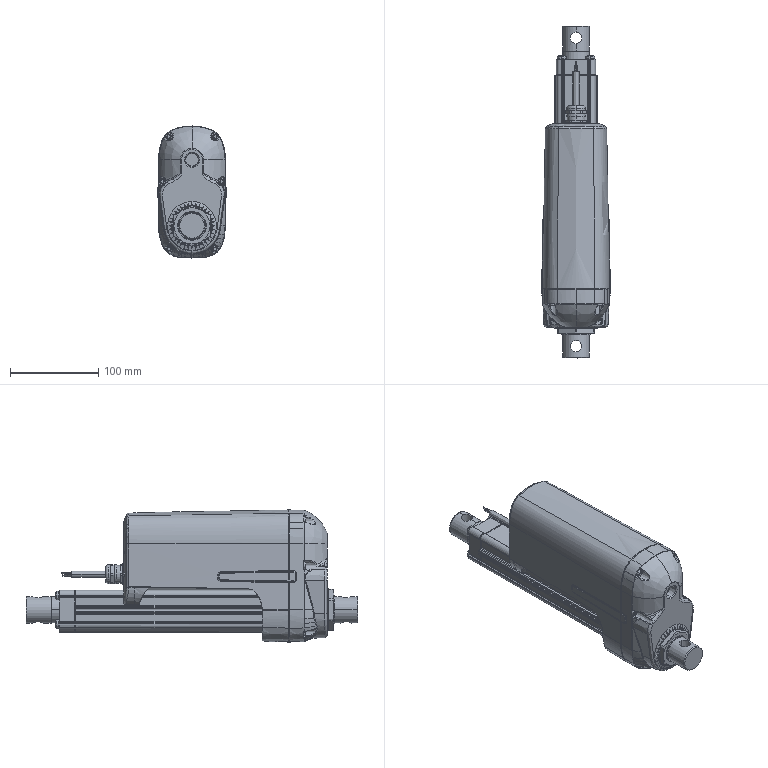Part | SolidWorks | 2 solids | 2355 faces | box 78.005 x 377.029 x 149.97 mm | volume 2205141 mm3 | cylinder 984 | plane 501 | spline 428 | torus 158 | cone 152 | sphere 132 | commonest cylinder face diameters 0.4 x290 1 x234 2 x69 1.3 x48 1.384 x42 1.7 x22